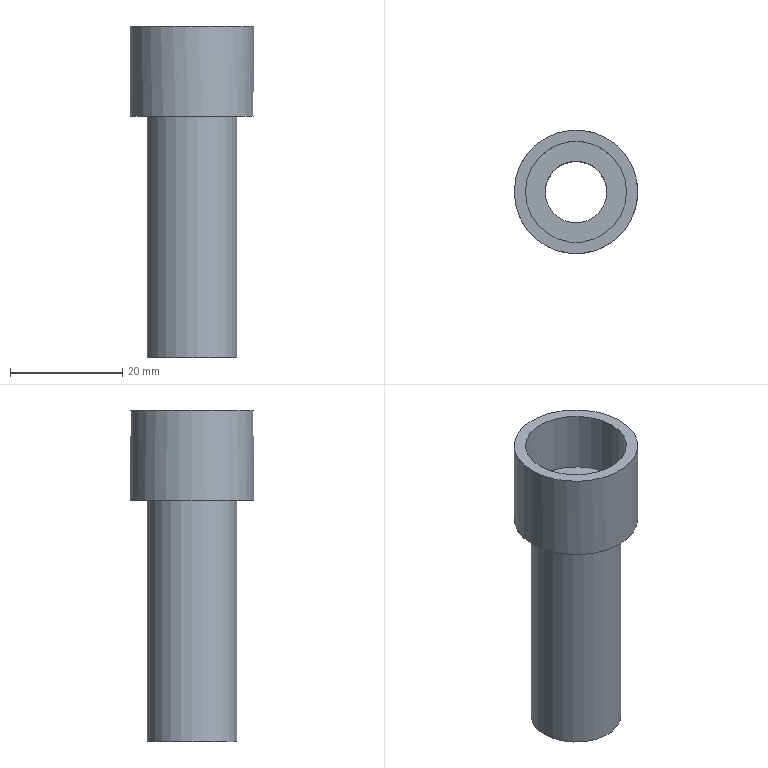Part | STEP file | lll_id282_x_t | 1 solid | 8 faces | box 22 x 22 x 59 mm | volume 7367 mm3 | plane 4 | cylinder 4 | commonest cylinder face diameters 11 x1 16 x1 18 x1 22 x1
STEP:
#1=CARTESIAN_POINT('',(-102.5,77.,95.5));
#2=VERTEX_POINT('',#1);
#3=CARTESIAN_POINT('',(-97.,77.,95.5));
#4=DIRECTION('',(0.,0.,-1.));
#5=DIRECTION('',(-1.,0.,0.));
#6=AXIS2_PLACEMENT_3D('',#3,#4,#5);
#7=CIRCLE('',#6,5.5);
#8=EDGE_CURVE('',#2,#2,#7,.T.);
#9=ORIENTED_EDGE('',*,*,#8,.F.);
#10=EDGE_LOOP('',(#9));
#11=FACE_BOUND('',#10,.T.);
#12=CARTESIAN_POINT('',(-89.,77.,95.5));
#13=VERTEX_POINT('',#12);
#14=CARTESIAN_POINT('',(-97.,77.,95.5));
#15=DIRECTION('',(0.,0.,1.));
#16=DIRECTION('',(1.,0.,0.));
#17=AXIS2_PLACEMENT_3D('',#14,#15,#16);
#18=CIRCLE('',#17,8.);
#19=EDGE_CURVE('',#13,#13,#18,.T.);
#20=ORIENTED_EDGE('',*,*,#19,.F.);
#21=EDGE_LOOP('',(#20));
#22=FACE_BOUND('',#21,.T.);
#23=CARTESIAN_POINT('',(-97.,77.,95.5));
#24=DIRECTION('',(0.,0.,-1.));
#25=DIRECTION('',(-1.,0.,0.));
#26=AXIS2_PLACEMENT_3D('',#23,#24,#25);
#27=PLANE('',#26);
#28=ADVANCED_FACE('',(#11,#22),#27,.T.);
#29=CARTESIAN_POINT('',(-105.,77.,138.5));
#30=VERTEX_POINT('',#29);
#31=CARTESIAN_POINT('',(-97.,77.,138.5));
#32=DIRECTION('',(0.,0.,1.));
#33=DIRECTION('',(-1.,0.,0.));
#34=AXIS2_PLACEMENT_3D('',#31,#32,#33);
#35=CIRCLE('',#34,8.);
#36=EDGE_CURVE('',#30,#30,#35,.T.);
#37=ORIENTED_EDGE('',*,*,#36,.F.);
#38=EDGE_LOOP('',(#37));
#39=FACE_BOUND('',#38,.T.);
#40=ORIENTED_EDGE('',*,*,#19,.T.);
#41=EDGE_LOOP('',(#40));
#42=FACE_BOUND('',#41,.T.);
#43=CARTESIAN_POINT('',(-97.,77.,95.5));
#44=DIRECTION('',(0.,0.,1.));
#45=DIRECTION('',(1.,0.,0.));
#46=AXIS2_PLACEMENT_3D('',#43,#44,#45);
#47=CYLINDRICAL_SURFACE('',#46,8.);
#48=ADVANCED_FACE('',(#39,#42),#47,.T.);
#49=ORIENTED_EDGE('',*,*,#36,.T.);
#50=EDGE_LOOP('',(#49));
#51=FACE_BOUND('',#50,.T.);
#52=CARTESIAN_POINT('',(-108.,77.,138.5));
#53=VERTEX_POINT('',#52);
#54=CARTESIAN_POINT('',(-97.,77.,138.5));
#55=DIRECTION('',(0.,0.,1.));
#56=DIRECTION('',(-1.,0.,0.));
#57=AXIS2_PLACEMENT_3D('',#54,#55,#56);
#58=CIRCLE('',#57,11.);
#59=EDGE_CURVE('',#53,#53,#58,.T.);
#60=ORIENTED_EDGE('',*,*,#59,.F.);
#61=EDGE_LOOP('',(#60));
#62=FACE_BOUND('',#61,.T.);
#63=CARTESIAN_POINT('',(-97.,77.,138.5));
#64=DIRECTION('',(0.,0.,-1.));
#65=DIRECTION('',(-1.,0.,0.));
#66=AXIS2_PLACEMENT_3D('',#63,#64,#65);
#67=PLANE('',#66);
#68=ADVANCED_FACE('',(#51,#62),#67,.T.);
#69=ORIENTED_EDGE('',*,*,#59,.T.);
#70=EDGE_LOOP('',(#69));
#71=FACE_BOUND('',#70,.T.);
#72=CARTESIAN_POINT('',(-86.,77.,154.5));
#73=VERTEX_POINT('',#72);
#74=CARTESIAN_POINT('',(-97.,77.,154.5));
#75=DIRECTION('',(0.,0.,-1.));
#76=DIRECTION('',(1.,0.,0.));
#77=AXIS2_PLACEMENT_3D('',#74,#75,#76);
#78=CIRCLE('',#77,11.);
#79=EDGE_CURVE('',#73,#73,#78,.T.);
#80=ORIENTED_EDGE('',*,*,#79,.T.);
#81=EDGE_LOOP('',(#80));
#82=FACE_BOUND('',#81,.T.);
#83=CARTESIAN_POINT('',(-97.,77.,142.5));
#84=DIRECTION('',(0.,0.,-1.));
#85=DIRECTION('',(-1.,0.,0.));
#86=AXIS2_PLACEMENT_3D('',#83,#84,#85);
#87=CYLINDRICAL_SURFACE('',#86,11.);
#88=ADVANCED_FACE('',(#71,#82),#87,.T.);
#89=CARTESIAN_POINT('',(-88.,77.,154.5));
#90=VERTEX_POINT('',#89);
#91=CARTESIAN_POINT('',(-97.,77.,154.5));
#92=DIRECTION('',(0.,0.,-1.));
#93=DIRECTION('',(1.,0.,0.));
#94=AXIS2_PLACEMENT_3D('',#91,#92,#93);
#95=CIRCLE('',#94,9.);
#96=EDGE_CURVE('',#90,#90,#95,.T.);
#97=ORIENTED_EDGE('',*,*,#96,.T.);
#98=EDGE_LOOP('',(#97));
#99=FACE_BOUND('',#98,.T.);
#100=ORIENTED_EDGE('',*,*,#79,.F.);
#101=EDGE_LOOP('',(#100));
#102=FACE_BOUND('',#101,.T.);
#103=CARTESIAN_POINT('',(-97.,77.,154.5));
#104=DIRECTION('',(0.,0.,1.));
#105=DIRECTION('',(1.,0.,0.));
#106=AXIS2_PLACEMENT_3D('',#103,#104,#105);
#107=PLANE('',#106);
#108=ADVANCED_FACE('',(#99,#102),#107,.T.);
#109=ORIENTED_EDGE('',*,*,#8,.T.);
#110=EDGE_LOOP('',(#109));
#111=FACE_BOUND('',#110,.T.);
#112=CARTESIAN_POINT('',(-102.5,77.,143.5));
#113=VERTEX_POINT('',#112);
#114=CARTESIAN_POINT('',(-97.,77.,143.5));
#115=DIRECTION('',(0.,0.,-1.));
#116=DIRECTION('',(-1.,0.,0.));
#117=AXIS2_PLACEMENT_3D('',#114,#115,#116);
#118=CIRCLE('',#117,5.5);
#119=EDGE_CURVE('',#113,#113,#118,.T.);
#120=ORIENTED_EDGE('',*,*,#119,.F.);
#121=EDGE_LOOP('',(#120));
#122=FACE_BOUND('',#121,.T.);
#123=CARTESIAN_POINT('',(-97.,77.,-157.5));
#124=DIRECTION('',(0.,0.,-1.));
#125=DIRECTION('',(-1.,0.,0.));
#126=AXIS2_PLACEMENT_3D('',#123,#124,#125);
#127=CYLINDRICAL_SURFACE('',#126,5.5);
#128=ADVANCED_FACE('',(#111,#122),#127,.F.);
#129=ORIENTED_EDGE('',*,*,#119,.T.);
#130=EDGE_LOOP('',(#129));
#131=FACE_BOUND('',#130,.T.);
#132=CARTESIAN_POINT('',(-106.,77.,143.5));
#133=VERTEX_POINT('',#132);
#134=CARTESIAN_POINT('',(-97.,77.,143.5));
#135=DIRECTION('',(0.,0.,-1.));
#136=DIRECTION('',(-1.,0.,0.));
#137=AXIS2_PLACEMENT_3D('',#134,#135,#136);
#138=CIRCLE('',#137,9.);
#139=EDGE_CURVE('',#133,#133,#138,.T.);
#140=ORIENTED_EDGE('',*,*,#139,.F.);
#141=EDGE_LOOP('',(#140));
#142=FACE_BOUND('',#141,.T.);
#143=CARTESIAN_POINT('',(-97.,77.,143.5));
#144=DIRECTION('',(0.,0.,-1.));
#145=DIRECTION('',(-1.,0.,0.));
#146=AXIS2_PLACEMENT_3D('',#143,#144,#145);
#147=PLANE('',#146);
#148=ADVANCED_FACE('',(#131,#142),#147,.F.);
#149=ORIENTED_EDGE('',*,*,#139,.T.);
#150=EDGE_LOOP('',(#149));
#151=FACE_BOUND('',#150,.T.);
#152=ORIENTED_EDGE('',*,*,#96,.F.);
#153=EDGE_LOOP('',(#152));
#154=FACE_BOUND('',#153,.T.);
#155=CARTESIAN_POINT('',(-97.,77.,142.5));
#156=DIRECTION('',(0.,0.,-1.));
#157=DIRECTION('',(-1.,0.,0.));
#158=AXIS2_PLACEMENT_3D('',#155,#156,#157);
#159=CYLINDRICAL_SURFACE('',#158,9.);
#160=ADVANCED_FACE('',(#151,#154),#159,.F.);
#161=CLOSED_SHELL('',(#28,#48,#68,#88,#108,#128,#148,#160));
#162=MANIFOLD_SOLID_BREP('',#161);
#163=(LENGTH_UNIT()NAMED_UNIT(*)SI_UNIT(.MILLI.,.METRE.));
#164=UNCERTAINTY_MEASURE_WITH_UNIT(LENGTH_MEASURE(0.00002),#163,'','');
#165=(NAMED_UNIT(*)PLANE_ANGLE_UNIT()SI_UNIT($,.RADIAN.));
#166=PLANE_ANGLE_MEASURE_WITH_UNIT(PLANE_ANGLE_MEASURE(0.01745),#165);
#167=DIMENSIONAL_EXPONENTS(0.,0.,0.,0.,0.,0.,0.);
#168=(CONVERSION_BASED_UNIT('DEGREE',#166)NAMED_UNIT(#167)PLANE_ANGLE_UNIT());
#169=(NAMED_UNIT(*)SI_UNIT($,.STERADIAN.)SOLID_ANGLE_UNIT());
#170=(GEOMETRIC_REPRESENTATION_CONTEXT(3)GLOBAL_UNCERTAINTY_ASSIGNED_CONTEXT((#164))GLOBAL_UNIT_ASSIGNED_CONTEXT((#163,#168,#169))REPRESENTATION_CONTEXT('',''));
#171=ADVANCED_BREP_SHAPE_REPRESENTATION('',(#162),#170);